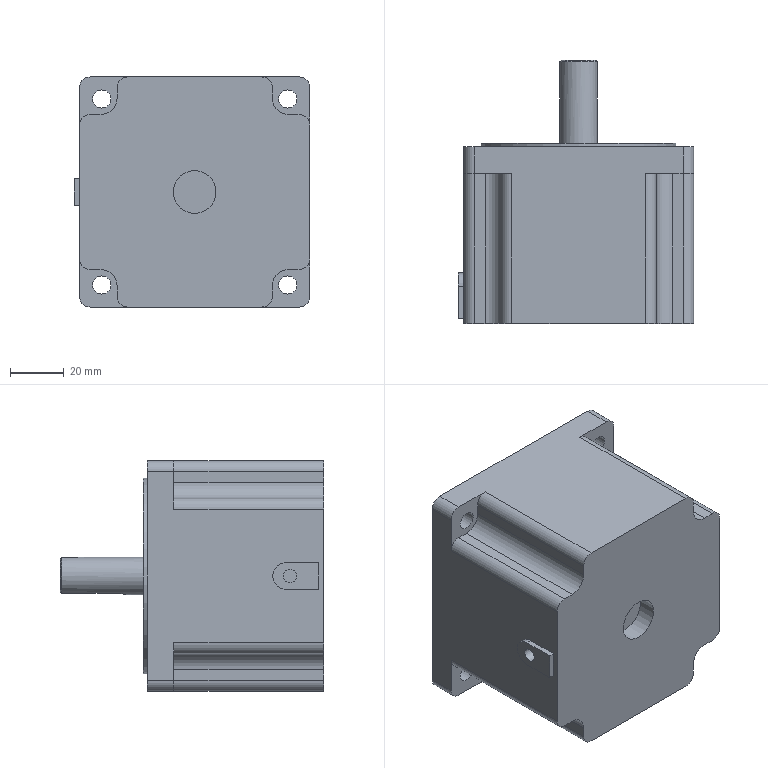Part | NX | features BREP 1 | 1 solid | 58 faces | box 88 x 98.4 x 86 mm | volume 447991 mm3 | plane 30 | cylinder 26 | cone 2 | commonest cylinder face diameters 8 x12 6.8 x4 12 x4 5 x2 10 x1 14 x1